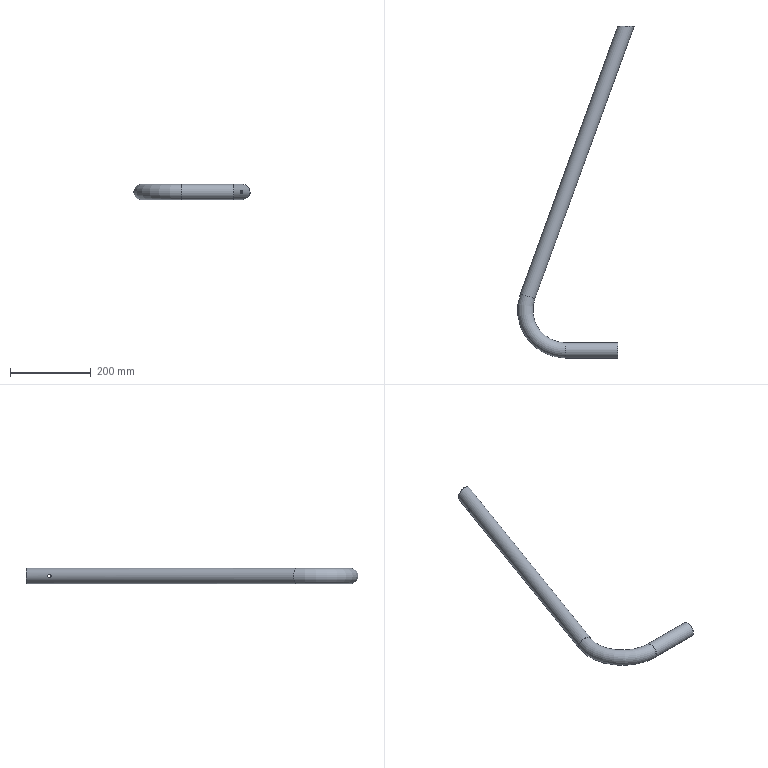Part | STEP file | 6151401 | 1 solid | 10 faces | box 289.236 x 823.315 x 38.1 mm | volume 178322 mm3 | cylinder 6 | torus 2 | plane 2 | commonest cylinder face diameters 9 x2 35.1 x2 38.1 x2
STEP:
#1=CARTESIAN_POINT('',(-23.107,741.765,0.));
#2=VERTEX_POINT('',#1);
#3=CARTESIAN_POINT('',(-23.107,741.765,0.));
#4=CARTESIAN_POINT('',(-23.107,741.765,-0.3084));
#5=CARTESIAN_POINT('',(-23.088,741.797,-0.6103));
#6=CARTESIAN_POINT('',(-23.013,741.918,-1.202));
#7=CARTESIAN_POINT('',(-22.958,742.01,-1.494));
#8=CARTESIAN_POINT('',(-22.819,742.243,-2.039));
#9=CARTESIAN_POINT('',(-22.735,742.384,-2.296));
#10=CARTESIAN_POINT('',(-22.546,742.715,-2.78));
#11=CARTESIAN_POINT('',(-22.443,742.899,-3.));
#12=CARTESIAN_POINT('',(-22.223,743.303,-3.399));
#13=CARTESIAN_POINT('',(-22.106,743.525,-3.581));
#14=CARTESIAN_POINT('',(-21.869,743.992,-3.894));
#15=CARTESIAN_POINT('',(-21.749,744.237,-4.027));
#16=CARTESIAN_POINT('',(-21.51,744.753,-4.248));
#17=CARTESIAN_POINT('',(-21.389,745.024,-4.335));
#18=CARTESIAN_POINT('',(-21.159,745.573,-4.455));
#19=CARTESIAN_POINT('',(-21.048,745.853,-4.49));
#20=CARTESIAN_POINT('',(-20.836,746.425,-4.506));
#21=CARTESIAN_POINT('',(-20.735,746.717,-4.487));
#22=CARTESIAN_POINT('',(-20.551,747.287,-4.392));
#23=CARTESIAN_POINT('',(-20.468,747.569,-4.317));
#24=CARTESIAN_POINT('',(-20.354,747.985,-4.161));
#25=CARTESIAN_POINT('',(-20.318,748.123,-4.101));
#26=CARTESIAN_POINT('',(-20.251,748.39,-3.97));
#27=CARTESIAN_POINT('',(-20.22,748.52,-3.897));
#28=CARTESIAN_POINT('',(-20.133,748.899,-3.661));
#29=CARTESIAN_POINT('',(-20.084,749.138,-3.477));
#30=CARTESIAN_POINT('',(-20.001,749.581,-3.058));
#31=CARTESIAN_POINT('',(-19.968,749.778,-2.829));
#32=CARTESIAN_POINT('',(-19.913,750.125,-2.333));
#33=CARTESIAN_POINT('',(-19.892,750.276,-2.062));
#34=CARTESIAN_POINT('',(-19.86,750.518,-1.503));
#35=CARTESIAN_POINT('',(-19.849,750.609,-1.213));
#36=CARTESIAN_POINT('',(-19.838,750.702,-0.7642));
#37=CARTESIAN_POINT('',(-19.836,750.726,-0.6113));
#38=CARTESIAN_POINT('',(-19.832,750.757,-0.3069));
#39=CARTESIAN_POINT('',(-19.831,750.765,-0.1548));
#40=CARTESIAN_POINT('',(-19.831,750.765,0.301));
#41=CARTESIAN_POINT('',(-19.835,750.735,0.6059));
#42=CARTESIAN_POINT('',(-19.849,750.611,1.208));
#43=CARTESIAN_POINT('',(-19.86,750.52,1.498));
#44=CARTESIAN_POINT('',(-19.892,750.28,2.056));
#45=CARTESIAN_POINT('',(-19.913,750.129,2.327));
#46=CARTESIAN_POINT('',(-19.967,749.782,2.824));
#47=CARTESIAN_POINT('',(-20.,749.585,3.053));
#48=CARTESIAN_POINT('',(-20.083,749.145,3.471));
#49=CARTESIAN_POINT('',(-20.132,748.904,3.658));
#50=CARTESIAN_POINT('',(-20.248,748.398,3.974));
#51=CARTESIAN_POINT('',(-20.315,748.128,4.107));
#52=CARTESIAN_POINT('',(-20.466,747.572,4.316));
#53=CARTESIAN_POINT('',(-20.55,747.29,4.391));
#54=CARTESIAN_POINT('',(-20.735,746.717,4.487));
#55=CARTESIAN_POINT('',(-20.836,746.424,4.506));
#56=CARTESIAN_POINT('',(-21.048,745.853,4.49));
#57=CARTESIAN_POINT('',(-21.159,745.572,4.455));
#58=CARTESIAN_POINT('',(-21.391,745.019,4.333));
#59=CARTESIAN_POINT('',(-21.511,744.749,4.246));
#60=CARTESIAN_POINT('',(-21.75,744.235,4.026));
#61=CARTESIAN_POINT('',(-21.87,743.989,3.892));
#62=CARTESIAN_POINT('',(-22.109,743.519,3.576));
#63=CARTESIAN_POINT('',(-22.224,743.301,3.397));
#64=CARTESIAN_POINT('',(-22.443,742.899,2.999));
#65=CARTESIAN_POINT('',(-22.546,742.715,2.781));
#66=CARTESIAN_POINT('',(-22.735,742.385,2.297));
#67=CARTESIAN_POINT('',(-22.818,742.243,2.04));
#68=CARTESIAN_POINT('',(-22.956,742.012,1.499));
#69=CARTESIAN_POINT('',(-23.012,741.921,1.211));
#70=CARTESIAN_POINT('',(-23.087,741.797,0.6128));
#71=CARTESIAN_POINT('',(-23.107,741.765,0.3084));
#72=CARTESIAN_POINT('',(-23.107,741.765,0.));
#73=B_SPLINE_CURVE_WITH_KNOTS('',3,(#3,#4,#5,#6,#7,#8,#9,#10,#11,#12,#13,#14,#15,#16,#17,#18,#19,#20,#21,#22,#23,#24,#25,#26,#27,#28,#29,#30,#31,#32,#33,#34,#35,#36,#37,#38,#39,#40,#41,#42,#43,#44,#45,#46,#47,#48,#49,#50,#51,#52,#53,#54,#55,#56,#57,#58,#59,#60,#61,#62,#63,#64,#65,#66,#67,#68,#69,#70,#71,#72),.UNSPECIFIED.,.T.,.F.,(4,2,2,2,2,2,2,2,2,2,2,2,2,2,2,2,2,2,2,2,2,2,2,2,2,2,2,2,2,2,2,2,2,2,4),(0.,0.0009109,0.001822,0.002733,0.003644,0.004555,0.005465,0.006376,0.007287,0.008198,0.009109,0.009564,0.01002,0.01093,0.01184,0.01275,0.01366,0.01412,0.01457,0.01549,0.0164,0.01731,0.01822,0.01913,0.02004,0.02095,0.02186,0.02277,0.02368,0.02459,0.02551,0.02642,0.02733,0.02824,0.02915),.UNSPECIFIED.);
#74=EDGE_CURVE('',#2,#2,#73,.T.);
#75=ORIENTED_EDGE('',*,*,#74,.T.);
#76=EDGE_LOOP('',(#75));
#77=FACE_BOUND('',#76,.T.);
#78=CARTESIAN_POINT('',(17.438,741.765,0.));
#79=VERTEX_POINT('',#78);
#80=CARTESIAN_POINT('',(17.438,741.765,0.));
#81=CARTESIAN_POINT('',(17.438,741.765,0.3079));
#82=CARTESIAN_POINT('',(17.442,741.796,0.6104));
#83=CARTESIAN_POINT('',(17.456,741.919,1.205));
#84=CARTESIAN_POINT('',(17.467,742.012,1.501));
#85=CARTESIAN_POINT('',(17.499,742.253,2.06));
#86=CARTESIAN_POINT('',(17.52,742.4,2.325));
#87=CARTESIAN_POINT('',(17.574,742.748,2.824));
#88=CARTESIAN_POINT('',(17.608,742.949,3.057));
#89=CARTESIAN_POINT('',(17.69,743.385,3.471));
#90=CARTESIAN_POINT('',(17.739,743.624,3.656));
#91=CARTESIAN_POINT('',(17.855,744.135,3.976));
#92=CARTESIAN_POINT('',(17.922,744.402,4.107));
#93=CARTESIAN_POINT('',(18.072,744.953,4.314));
#94=CARTESIAN_POINT('',(18.157,745.241,4.391));
#95=CARTESIAN_POINT('',(18.342,745.814,4.487));
#96=CARTESIAN_POINT('',(18.441,746.101,4.506));
#97=CARTESIAN_POINT('',(18.653,746.674,4.491));
#98=CARTESIAN_POINT('',(18.766,746.958,4.455));
#99=CARTESIAN_POINT('',(18.997,747.507,4.334));
#100=CARTESIAN_POINT('',(19.115,747.774,4.249));
#101=CARTESIAN_POINT('',(19.478,748.554,3.916));
#102=CARTESIAN_POINT('',(19.717,749.019,3.605));
#103=CARTESIAN_POINT('',(20.049,749.631,3.001));
#104=CARTESIAN_POINT('',(20.152,749.814,2.782));
#105=CARTESIAN_POINT('',(20.339,750.139,2.307));
#106=CARTESIAN_POINT('',(20.423,750.282,2.05));
#107=CARTESIAN_POINT('',(20.563,750.518,1.501));
#108=CARTESIAN_POINT('',(20.618,750.608,1.216));
#109=CARTESIAN_POINT('',(20.674,750.7,0.7752));
#110=CARTESIAN_POINT('',(20.689,750.724,0.6257));
#111=CARTESIAN_POINT('',(20.709,750.756,0.3212));
#112=CARTESIAN_POINT('',(20.714,750.765,0.1668));
#113=CARTESIAN_POINT('',(20.715,750.766,-0.2909));
#114=CARTESIAN_POINT('',(20.696,750.736,-0.5928));
#115=CARTESIAN_POINT('',(20.622,750.616,-1.191));
#116=CARTESIAN_POINT('',(20.568,750.525,-1.48));
#117=CARTESIAN_POINT('',(20.429,750.294,-2.027));
#118=CARTESIAN_POINT('',(20.345,750.15,-2.289));
#119=CARTESIAN_POINT('',(20.158,749.824,-2.77));
#120=CARTESIAN_POINT('',(20.054,749.64,-2.99));
#121=CARTESIAN_POINT('',(19.833,749.233,-3.395));
#122=CARTESIAN_POINT('',(19.717,749.014,-3.574));
#123=CARTESIAN_POINT('',(19.481,748.549,-3.888));
#124=CARTESIAN_POINT('',(19.36,748.3,-4.023));
#125=CARTESIAN_POINT('',(19.119,747.783,-4.246));
#126=CARTESIAN_POINT('',(19.,747.516,-4.332));
#127=CARTESIAN_POINT('',(18.77,746.968,-4.454));
#128=CARTESIAN_POINT('',(18.657,746.682,-4.49));
#129=CARTESIAN_POINT('',(18.444,746.109,-4.506));
#130=CARTESIAN_POINT('',(18.345,745.823,-4.488));
#131=CARTESIAN_POINT('',(18.161,745.252,-4.394));
#132=CARTESIAN_POINT('',(18.075,744.964,-4.318));
#133=CARTESIAN_POINT('',(17.924,744.41,-4.11));
#134=CARTESIAN_POINT('',(17.857,744.144,-3.98));
#135=CARTESIAN_POINT('',(17.741,743.636,-3.665));
#136=CARTESIAN_POINT('',(17.691,743.393,-3.477));
#137=CARTESIAN_POINT('',(17.609,742.955,-3.063));
#138=CARTESIAN_POINT('',(17.575,742.757,-2.834));
#139=CARTESIAN_POINT('',(17.52,742.405,-2.333));
#140=CARTESIAN_POINT('',(17.499,742.256,-2.065));
#141=CARTESIAN_POINT('',(17.468,742.015,-1.508));
#142=CARTESIAN_POINT('',(17.456,741.921,-1.214));
#143=CARTESIAN_POINT('',(17.442,741.797,-0.6129));
#144=CARTESIAN_POINT('',(17.438,741.765,-0.3079));
#145=CARTESIAN_POINT('',(17.438,741.765,0.));
#146=B_SPLINE_CURVE_WITH_KNOTS('',3,(#80,#81,#82,#83,#84,#85,#86,#87,#88,#89,#90,#91,#92,#93,#94,#95,#96,#97,#98,#99,#100,#101,#102,#103,#104,#105,#106,#107,#108,#109,#110,#111,#112,#113,#114,#115,#116,#117,#118,#119,#120,#121,#122,#123,#124,#125,#126,#127,#128,#129,#130,#131,#132,#133,#134,#135,#136,#137,#138,#139,#140,#141,#142,#143,#144,#145),.UNSPECIFIED.,.T.,.F.,(4,2,2,2,2,2,2,2,2,2,2,2,2,2,2,2,2,2,2,2,2,2,2,2,2,2,2,2,2,2,2,2,4),(0.,0.0009106,0.001821,0.002732,0.003642,0.004553,0.005464,0.006374,0.007285,0.008196,0.009106,0.01093,0.01184,0.01275,0.01366,0.01411,0.01457,0.01548,0.01639,0.0173,0.01821,0.01912,0.02003,0.02094,0.02185,0.02277,0.02368,0.02459,0.0255,0.02641,0.02732,0.02823,0.02914),.UNSPECIFIED.);
#147=EDGE_CURVE('',#79,#79,#146,.T.);
#148=ORIENTED_EDGE('',*,*,#147,.T.);
#149=EDGE_LOOP('',(#148));
#150=FACE_BOUND('',#149,.T.);
#151=CARTESIAN_POINT('',(40.186,804.265,0.));
#152=VERTEX_POINT('',#151);
#153=CARTESIAN_POINT('',(40.186,804.265,0.));
#154=CARTESIAN_POINT('',(40.186,804.265,38.1));
#155=CARTESIAN_POINT('',(-0.3588,804.265,38.1));
#156=CARTESIAN_POINT('',(-0.3588,804.265,0.));
#157=CARTESIAN_POINT('',(-0.3588,804.265,-38.1));
#158=CARTESIAN_POINT('',(40.186,804.265,-38.1));
#159=CARTESIAN_POINT('',(40.186,804.265,0.));
#160=(BOUNDED_CURVE()B_SPLINE_CURVE(3,(#153,#154,#155,#156,#157,#158,#159),.UNSPECIFIED.,.T.,.F.)B_SPLINE_CURVE_WITH_KNOTS((4,3,4),(0.,3.142,6.283),.UNSPECIFIED.)CURVE()GEOMETRIC_REPRESENTATION_ITEM()RATIONAL_B_SPLINE_CURVE((1.,0.3333,0.3333,1.,0.3333,0.3333,1.))REPRESENTATION_ITEM(''));
#161=EDGE_CURVE('',#152,#152,#160,.T.);
#162=ORIENTED_EDGE('',*,*,#161,.T.);
#163=EDGE_LOOP('',(#162));
#164=FACE_OUTER_BOUND('',#163,.T.);
#165=CARTESIAN_POINT('',(-223.969,134.202,-19.05));
#166=VERTEX_POINT('',#165);
#167=CARTESIAN_POINT('',(-223.969,134.202,0.));
#168=DIRECTION('',(-0.342,-0.9397,0.));
#169=DIRECTION('',(0.,0.,-1.));
#170=AXIS2_PLACEMENT_3D('',#167,#168,#169);
#171=CIRCLE('',#170,19.05);
#172=EDGE_CURVE('',#166,#166,#171,.T.);
#173=ORIENTED_EDGE('',*,*,#172,.F.);
#174=EDGE_LOOP('',(#173));
#175=FACE_OUTER_BOUND('',#174,.T.);
#176=CARTESIAN_POINT('',(-223.969,134.202,0.));
#177=DIRECTION('',(0.342,0.9397,0.));
#178=DIRECTION('',(-0.9397,0.342,0.));
#179=AXIS2_PLACEMENT_3D('',#176,#177,#178);
#180=CYLINDRICAL_SURFACE('',#179,19.05);
#181=ADVANCED_FACE('',(#77,#150,#164,#175),#180,.T.);
#182=CARTESIAN_POINT('',(-21.511,741.765,0.));
#183=VERTEX_POINT('',#182);
#184=CARTESIAN_POINT('',(-21.511,741.765,0.));
#185=CARTESIAN_POINT('',(-21.511,741.765,-0.3086));
#186=CARTESIAN_POINT('',(-21.491,741.797,-0.6106));
#187=CARTESIAN_POINT('',(-21.414,741.918,-1.202));
#188=CARTESIAN_POINT('',(-21.356,742.01,-1.494));
#189=CARTESIAN_POINT('',(-21.213,742.243,-2.039));
#190=CARTESIAN_POINT('',(-21.127,742.384,-2.296));
#191=CARTESIAN_POINT('',(-20.932,742.713,-2.778));
#192=CARTESIAN_POINT('',(-20.826,742.897,-2.997));
#193=CARTESIAN_POINT('',(-20.601,743.299,-3.396));
#194=CARTESIAN_POINT('',(-20.481,743.52,-3.577));
#195=CARTESIAN_POINT('',(-20.239,743.985,-3.89));
#196=CARTESIAN_POINT('',(-20.117,744.229,-4.023));
#197=CARTESIAN_POINT('',(-19.873,744.743,-4.244));
#198=CARTESIAN_POINT('',(-19.751,745.014,-4.332));
#199=CARTESIAN_POINT('',(-19.518,745.562,-4.454));
#200=CARTESIAN_POINT('',(-19.406,745.841,-4.489));
#201=CARTESIAN_POINT('',(-19.193,746.413,-4.507));
#202=CARTESIAN_POINT('',(-19.092,746.705,-4.488));
#203=CARTESIAN_POINT('',(-18.91,747.277,-4.394));
#204=CARTESIAN_POINT('',(-18.828,747.559,-4.32));
#205=CARTESIAN_POINT('',(-18.717,747.976,-4.165));
#206=CARTESIAN_POINT('',(-18.682,748.115,-4.105));
#207=CARTESIAN_POINT('',(-18.617,748.383,-3.973));
#208=CARTESIAN_POINT('',(-18.588,748.513,-3.901));
#209=CARTESIAN_POINT('',(-18.505,748.894,-3.665));
#210=CARTESIAN_POINT('',(-18.459,749.133,-3.481));
#211=CARTESIAN_POINT('',(-18.382,749.578,-3.061));
#212=CARTESIAN_POINT('',(-18.352,749.775,-2.832));
#213=CARTESIAN_POINT('',(-18.304,750.124,-2.335));
#214=CARTESIAN_POINT('',(-18.286,750.275,-2.065));
#215=CARTESIAN_POINT('',(-18.259,750.517,-1.505));
#216=CARTESIAN_POINT('',(-18.25,750.609,-1.215));
#217=CARTESIAN_POINT('',(-18.238,750.733,-0.6156));
#218=CARTESIAN_POINT('',(-18.235,750.765,-0.3081));
#219=CARTESIAN_POINT('',(-18.235,750.765,0.2999));
#220=CARTESIAN_POINT('',(-18.238,750.735,0.6057));
#221=CARTESIAN_POINT('',(-18.25,750.611,1.207));
#222=CARTESIAN_POINT('',(-18.259,750.52,1.497));
#223=CARTESIAN_POINT('',(-18.285,750.279,2.056));
#224=CARTESIAN_POINT('',(-18.304,750.128,2.328));
#225=CARTESIAN_POINT('',(-18.352,749.781,2.826));
#226=CARTESIAN_POINT('',(-18.381,749.583,3.055));
#227=CARTESIAN_POINT('',(-18.458,749.142,3.474));
#228=CARTESIAN_POINT('',(-18.504,748.9,3.66));
#229=CARTESIAN_POINT('',(-18.613,748.393,3.977));
#230=CARTESIAN_POINT('',(-18.678,748.122,4.11));
#231=CARTESIAN_POINT('',(-18.826,747.565,4.318));
#232=CARTESIAN_POINT('',(-18.908,747.282,4.393));
#233=CARTESIAN_POINT('',(-19.091,746.707,4.488));
#234=CARTESIAN_POINT('',(-19.192,746.414,4.507));
#235=CARTESIAN_POINT('',(-19.405,745.844,4.489));
#236=CARTESIAN_POINT('',(-19.517,745.563,4.454));
#237=CARTESIAN_POINT('',(-19.752,745.01,4.331));
#238=CARTESIAN_POINT('',(-19.874,744.741,4.243));
#239=CARTESIAN_POINT('',(-20.117,744.229,4.023));
#240=CARTESIAN_POINT('',(-20.24,743.984,3.889));
#241=CARTESIAN_POINT('',(-20.483,743.515,3.573));
#242=CARTESIAN_POINT('',(-20.601,743.298,3.395));
#243=CARTESIAN_POINT('',(-20.825,742.898,2.998));
#244=CARTESIAN_POINT('',(-20.931,742.714,2.779));
#245=CARTESIAN_POINT('',(-21.126,742.384,2.297));
#246=CARTESIAN_POINT('',(-21.212,742.244,2.04));
#247=CARTESIAN_POINT('',(-21.356,742.011,1.496));
#248=CARTESIAN_POINT('',(-21.413,741.919,1.204));
#249=CARTESIAN_POINT('',(-21.491,741.797,0.6114));
#250=CARTESIAN_POINT('',(-21.511,741.765,0.3086));
#251=CARTESIAN_POINT('',(-21.511,741.765,0.));
#252=B_SPLINE_CURVE_WITH_KNOTS('',3,(#184,#185,#186,#187,#188,#189,#190,#191,#192,#193,#194,#195,#196,#197,#198,#199,#200,#201,#202,#203,#204,#205,#206,#207,#208,#209,#210,#211,#212,#213,#214,#215,#216,#217,#218,#219,#220,#221,#222,#223,#224,#225,#226,#227,#228,#229,#230,#231,#232,#233,#234,#235,#236,#237,#238,#239,#240,#241,#242,#243,#244,#245,#246,#247,#248,#249,#250,#251),.UNSPECIFIED.,.T.,.F.,(4,2,2,2,2,2,2,2,2,2,2,2,2,2,2,2,2,2,2,2,2,2,2,2,2,2,2,2,2,2,2,2,2,4),(0.,0.0009114,0.001823,0.002734,0.003646,0.004557,0.005468,0.00638,0.007291,0.008202,0.009114,0.009569,0.01003,0.01094,0.01185,0.01276,0.01367,0.01458,0.01549,0.0164,0.01732,0.01823,0.01914,0.02005,0.02096,0.02187,0.02278,0.0237,0.02461,0.02552,0.02643,0.02734,0.02825,0.02916),.UNSPECIFIED.);
#253=EDGE_CURVE('',#183,#183,#252,.T.);
#254=ORIENTED_EDGE('',*,*,#253,.F.);
#255=EDGE_LOOP('',(#254));
#256=FACE_BOUND('',#255,.T.);
#257=CARTESIAN_POINT('',(15.842,741.765,0.));
#258=VERTEX_POINT('',#257);
#259=CARTESIAN_POINT('',(15.842,741.765,0.));
#260=CARTESIAN_POINT('',(15.842,741.765,0.3081));
#261=CARTESIAN_POINT('',(15.845,741.797,0.6108));
#262=CARTESIAN_POINT('',(15.857,741.919,1.206));
#263=CARTESIAN_POINT('',(15.866,742.012,1.502));
#264=CARTESIAN_POINT('',(15.893,742.254,2.061));
#265=CARTESIAN_POINT('',(15.911,742.401,2.326));
#266=CARTESIAN_POINT('',(15.959,742.75,2.826));
#267=CARTESIAN_POINT('',(15.989,742.951,3.059));
#268=CARTESIAN_POINT('',(16.065,743.389,3.474));
#269=CARTESIAN_POINT('',(16.11,743.628,3.659));
#270=CARTESIAN_POINT('',(16.221,744.141,3.979));
#271=CARTESIAN_POINT('',(16.285,744.408,4.11));
#272=CARTESIAN_POINT('',(16.432,744.961,4.317));
#273=CARTESIAN_POINT('',(16.516,745.25,4.394));
#274=CARTESIAN_POINT('',(16.698,745.824,4.488));
#275=CARTESIAN_POINT('',(16.797,746.111,4.506));
#276=CARTESIAN_POINT('',(17.011,746.684,4.49));
#277=CARTESIAN_POINT('',(17.125,746.968,4.454));
#278=CARTESIAN_POINT('',(17.358,747.517,4.332));
#279=CARTESIAN_POINT('',(17.478,747.783,4.246));
#280=CARTESIAN_POINT('',(17.724,748.301,4.023));
#281=CARTESIAN_POINT('',(17.846,748.546,3.889));
#282=CARTESIAN_POINT('',(18.087,749.008,3.578));
#283=CARTESIAN_POINT('',(18.205,749.227,3.4));
#284=CARTESIAN_POINT('',(18.432,749.632,2.999));
#285=CARTESIAN_POINT('',(18.538,749.815,2.781));
#286=CARTESIAN_POINT('',(18.73,750.139,2.307));
#287=CARTESIAN_POINT('',(18.816,750.282,2.05));
#288=CARTESIAN_POINT('',(18.961,750.518,1.502));
#289=CARTESIAN_POINT('',(19.018,750.608,1.218));
#290=CARTESIAN_POINT('',(19.076,750.7,0.7769));
#291=CARTESIAN_POINT('',(19.091,750.724,0.6274));
#292=CARTESIAN_POINT('',(19.112,750.756,0.3228));
#293=CARTESIAN_POINT('',(19.117,750.765,0.1682));
#294=CARTESIAN_POINT('',(19.118,750.766,-0.2897));
#295=CARTESIAN_POINT('',(19.099,750.737,-0.5918));
#296=CARTESIAN_POINT('',(19.023,750.616,-1.19));
#297=CARTESIAN_POINT('',(18.966,750.526,-1.479));
#298=CARTESIAN_POINT('',(18.824,750.294,-2.026));
#299=CARTESIAN_POINT('',(18.737,750.151,-2.287));
#300=CARTESIAN_POINT('',(18.544,749.826,-2.767));
#301=CARTESIAN_POINT('',(18.438,749.643,-2.987));
#302=CARTESIAN_POINT('',(18.211,749.237,-3.391));
#303=CARTESIAN_POINT('',(18.092,749.019,-3.57));
#304=CARTESIAN_POINT('',(17.851,748.556,-3.884));
#305=CARTESIAN_POINT('',(17.727,748.308,-4.019));
#306=CARTESIAN_POINT('',(17.482,747.792,-4.242));
#307=CARTESIAN_POINT('',(17.362,747.527,-4.329));
#308=CARTESIAN_POINT('',(17.129,746.979,-4.452));
#309=CARTESIAN_POINT('',(17.015,746.694,-4.489));
#310=CARTESIAN_POINT('',(16.801,746.121,-4.507));
#311=CARTESIAN_POINT('',(16.702,745.835,-4.489));
#312=CARTESIAN_POINT('',(16.52,745.263,-4.396));
#313=CARTESIAN_POINT('',(16.435,744.974,-4.321));
#314=CARTESIAN_POINT('',(16.287,744.418,-4.114));
#315=CARTESIAN_POINT('',(16.224,744.151,-3.984));
#316=CARTESIAN_POINT('',(16.113,743.641,-3.668));
#317=CARTESIAN_POINT('',(16.066,743.397,-3.481));
#318=CARTESIAN_POINT('',(15.99,742.957,-3.066));
#319=CARTESIAN_POINT('',(15.96,742.759,-2.837));
#320=CARTESIAN_POINT('',(15.911,742.406,-2.335));
#321=CARTESIAN_POINT('',(15.893,742.257,-2.067));
#322=CARTESIAN_POINT('',(15.866,742.015,-1.509));
#323=CARTESIAN_POINT('',(15.857,741.921,-1.214));
#324=CARTESIAN_POINT('',(15.845,741.797,-0.6132));
#325=CARTESIAN_POINT('',(15.842,741.765,-0.3081));
#326=CARTESIAN_POINT('',(15.842,741.765,0.));
#327=B_SPLINE_CURVE_WITH_KNOTS('',3,(#259,#260,#261,#262,#263,#264,#265,#266,#267,#268,#269,#270,#271,#272,#273,#274,#275,#276,#277,#278,#279,#280,#281,#282,#283,#284,#285,#286,#287,#288,#289,#290,#291,#292,#293,#294,#295,#296,#297,#298,#299,#300,#301,#302,#303,#304,#305,#306,#307,#308,#309,#310,#311,#312,#313,#314,#315,#316,#317,#318,#319,#320,#321,#322,#323,#324,#325,#326),.UNSPECIFIED.,.T.,.F.,(4,2,2,2,2,2,2,2,2,2,2,2,2,2,2,2,2,2,2,2,2,2,2,2,2,2,2,2,2,2,2,2,2,4),(0.,0.0009111,0.001822,0.002733,0.003644,0.004556,0.005467,0.006378,0.007289,0.0082,0.009111,0.01002,0.01093,0.01184,0.01276,0.01367,0.01412,0.01458,0.01549,0.0164,0.01731,0.01822,0.01913,0.02004,0.02096,0.02187,0.02278,0.02369,0.0246,0.02551,0.02642,0.02733,0.02824,0.02916),.UNSPECIFIED.);
#328=EDGE_CURVE('',#258,#258,#327,.T.);
#329=ORIENTED_EDGE('',*,*,#328,.F.);
#330=EDGE_LOOP('',(#329));
#331=FACE_BOUND('',#330,.T.);
#332=CARTESIAN_POINT('',(38.59,804.265,0.));
#333=VERTEX_POINT('',#332);
#334=CARTESIAN_POINT('',(38.59,804.265,0.));
#335=CARTESIAN_POINT('',(38.59,804.265,35.1));
#336=CARTESIAN_POINT('',(1.237,804.265,35.1));
#337=CARTESIAN_POINT('',(1.237,804.265,0.));
#338=CARTESIAN_POINT('',(1.237,804.265,-35.1));
#339=CARTESIAN_POINT('',(38.59,804.265,-35.1));
#340=CARTESIAN_POINT('',(38.59,804.265,0.));
#341=(BOUNDED_CURVE()B_SPLINE_CURVE(3,(#334,#335,#336,#337,#338,#339,#340),.UNSPECIFIED.,.T.,.T.)B_SPLINE_CURVE_WITH_KNOTS((4,3,4),(0.,3.142,6.283),.UNSPECIFIED.)CURVE()GEOMETRIC_REPRESENTATION_ITEM()RATIONAL_B_SPLINE_CURVE((1.,0.3333,0.3333,1.,0.3333,0.3333,1.))REPRESENTATION_ITEM(''));
#342=EDGE_CURVE('',#333,#333,#341,.T.);
#343=ORIENTED_EDGE('',*,*,#342,.F.);
#344=EDGE_LOOP('',(#343));
#345=FACE_OUTER_BOUND('',#344,.T.);
#346=CARTESIAN_POINT('',(-223.969,134.202,-17.55));
#347=VERTEX_POINT('',#346);
#348=CARTESIAN_POINT('',(-223.969,134.202,0.));
#349=DIRECTION('',(-0.342,-0.9397,0.));
#350=DIRECTION('',(0.,0.,-1.));
#351=AXIS2_PLACEMENT_3D('',#348,#349,#350);
#352=CIRCLE('',#351,17.55);
#353=EDGE_CURVE('',#347,#347,#352,.T.);
#354=ORIENTED_EDGE('',*,*,#353,.T.);
#355=EDGE_LOOP('',(#354));
#356=FACE_OUTER_BOUND('',#355,.T.);
#357=CARTESIAN_POINT('',(-223.969,134.202,0.));
#358=DIRECTION('',(0.342,0.9397,0.));
#359=DIRECTION('',(-0.9397,0.342,0.));
#360=AXIS2_PLACEMENT_3D('',#357,#358,#359);
#361=CYLINDRICAL_SURFACE('',#360,17.55);
#362=ADVANCED_FACE('',(#256,#331,#345,#356),#361,.F.);
#363=CARTESIAN_POINT('',(-130.,0.,-19.05));
#364=VERTEX_POINT('',#363);
#365=CARTESIAN_POINT('',(-130.,0.,0.));
#366=DIRECTION('',(1.,0.,0.));
#367=DIRECTION('',(0.,0.,-1.));
#368=AXIS2_PLACEMENT_3D('',#365,#366,#367);
#369=CIRCLE('',#368,19.05);
#370=EDGE_CURVE('',#364,#364,#369,.T.);
#371=ORIENTED_EDGE('',*,*,#370,.F.);
#372=EDGE_LOOP('',(#371));
#373=FACE_OUTER_BOUND('',#372,.T.);
#374=ORIENTED_EDGE('',*,*,#172,.T.);
#375=EDGE_LOOP('',(#374));
#376=FACE_OUTER_BOUND('',#375,.T.);
#377=CARTESIAN_POINT('',(-130.,100.,0.));
#378=DIRECTION('',(0.,0.,-1.));
#379=DIRECTION('',(-1.,0.,0.));
#380=AXIS2_PLACEMENT_3D('',#377,#378,#379);
#381=TOROIDAL_SURFACE('',#380,100.,19.05);
#382=ADVANCED_FACE('',(#373,#376),#381,.T.);
#383=CARTESIAN_POINT('',(-130.,0.,-17.55));
#384=VERTEX_POINT('',#383);
#385=CARTESIAN_POINT('',(-130.,0.,0.));
#386=DIRECTION('',(1.,0.,0.));
#387=DIRECTION('',(0.,0.,-1.));
#388=AXIS2_PLACEMENT_3D('',#385,#386,#387);
#389=CIRCLE('',#388,17.55);
#390=EDGE_CURVE('',#384,#384,#389,.T.);
#391=ORIENTED_EDGE('',*,*,#390,.T.);
#392=EDGE_LOOP('',(#391));
#393=FACE_OUTER_BOUND('',#392,.T.);
#394=ORIENTED_EDGE('',*,*,#353,.F.);
#395=EDGE_LOOP('',(#394));
#396=FACE_OUTER_BOUND('',#395,.T.);
#397=CARTESIAN_POINT('',(-130.,100.,0.));
#398=DIRECTION('',(0.,0.,-1.));
#399=DIRECTION('',(-1.,0.,0.));
#400=AXIS2_PLACEMENT_3D('',#397,#398,#399);
#401=TOROIDAL_SURFACE('',#400,100.,17.55);
#402=ADVANCED_FACE('',(#393,#396),#401,.F.);
#403=ORIENTED_EDGE('',*,*,#390,.F.);
#404=EDGE_LOOP('',(#403));
#405=FACE_OUTER_BOUND('',#404,.T.);
#406=CARTESIAN_POINT('',(0.,0.,-17.55));
#407=VERTEX_POINT('',#406);
#408=CARTESIAN_POINT('',(0.,0.,0.));
#409=DIRECTION('',(1.,0.,0.));
#410=DIRECTION('',(0.,0.,-1.));
#411=AXIS2_PLACEMENT_3D('',#408,#409,#410);
#412=CIRCLE('',#411,17.55);
#413=EDGE_CURVE('',#407,#407,#412,.T.);
#414=ORIENTED_EDGE('',*,*,#413,.T.);
#415=EDGE_LOOP('',(#414));
#416=FACE_OUTER_BOUND('',#415,.T.);
#417=CARTESIAN_POINT('',(-130.,0.,0.));
#418=DIRECTION('',(1.,0.,0.));
#419=DIRECTION('',(0.,0.,-1.));
#420=AXIS2_PLACEMENT_3D('',#417,#418,#419);
#421=CYLINDRICAL_SURFACE('',#420,17.55);
#422=ADVANCED_FACE('',(#405,#416),#421,.F.);
#423=ORIENTED_EDGE('',*,*,#370,.T.);
#424=EDGE_LOOP('',(#423));
#425=FACE_OUTER_BOUND('',#424,.T.);
#426=CARTESIAN_POINT('',(0.,0.,-19.05));
#427=VERTEX_POINT('',#426);
#428=CARTESIAN_POINT('',(0.,0.,0.));
#429=DIRECTION('',(1.,0.,0.));
#430=DIRECTION('',(0.,0.,-1.));
#431=AXIS2_PLACEMENT_3D('',#428,#429,#430);
#432=CIRCLE('',#431,19.05);
#433=EDGE_CURVE('',#427,#427,#432,.T.);
#434=ORIENTED_EDGE('',*,*,#433,.F.);
#435=EDGE_LOOP('',(#434));
#436=FACE_OUTER_BOUND('',#435,.T.);
#437=CARTESIAN_POINT('',(-130.,0.,0.));
#438=DIRECTION('',(1.,0.,0.));
#439=DIRECTION('',(0.,0.,-1.));
#440=AXIS2_PLACEMENT_3D('',#437,#438,#439);
#441=CYLINDRICAL_SURFACE('',#440,19.05);
#442=ADVANCED_FACE('',(#425,#436),#441,.T.);
#443=ORIENTED_EDGE('',*,*,#413,.F.);
#444=EDGE_LOOP('',(#443));
#445=FACE_BOUND('',#444,.T.);
#446=ORIENTED_EDGE('',*,*,#433,.T.);
#447=EDGE_LOOP('',(#446));
#448=FACE_OUTER_BOUND('',#447,.T.);
#449=CARTESIAN_POINT('',(0.,0.,0.));
#450=DIRECTION('',(1.,0.,0.));
#451=DIRECTION('',(0.,0.,-1.));
#452=AXIS2_PLACEMENT_3D('',#449,#450,#451);
#453=PLANE('',#452);
#454=ADVANCED_FACE('',(#445,#448),#453,.T.);
#455=ORIENTED_EDGE('',*,*,#342,.T.);
#456=EDGE_LOOP('',(#455));
#457=FACE_BOUND('',#456,.T.);
#458=ORIENTED_EDGE('',*,*,#161,.F.);
#459=EDGE_LOOP('',(#458));
#460=FACE_OUTER_BOUND('',#459,.T.);
#461=CARTESIAN_POINT('',(40.186,804.265,1131.022));
#462=DIRECTION('',(0.,-1.,0.));
#463=DIRECTION('',(0.,0.,-1.));
#464=AXIS2_PLACEMENT_3D('',#461,#462,#463);
#465=PLANE('',#464);
#466=ADVANCED_FACE('',(#457,#460),#465,.F.);
#467=ORIENTED_EDGE('',*,*,#328,.T.);
#468=EDGE_LOOP('',(#467));
#469=FACE_OUTER_BOUND('',#468,.T.);
#470=ORIENTED_EDGE('',*,*,#147,.F.);
#471=EDGE_LOOP('',(#470));
#472=FACE_OUTER_BOUND('',#471,.T.);
#473=CARTESIAN_POINT('',(92.51,746.265,0.));
#474=DIRECTION('',(-1.,0.,0.));
#475=DIRECTION('',(0.,-1.,0.));
#476=AXIS2_PLACEMENT_3D('',#473,#474,#475);
#477=CYLINDRICAL_SURFACE('',#476,4.5);
#478=ADVANCED_FACE('',(#469,#472),#477,.F.);
#479=ORIENTED_EDGE('',*,*,#253,.T.);
#480=EDGE_LOOP('',(#479));
#481=FACE_OUTER_BOUND('',#480,.T.);
#482=ORIENTED_EDGE('',*,*,#74,.F.);
#483=EDGE_LOOP('',(#482));
#484=FACE_OUTER_BOUND('',#483,.T.);
#485=CARTESIAN_POINT('',(92.51,746.265,0.));
#486=DIRECTION('',(-1.,0.,0.));
#487=DIRECTION('',(0.,-1.,0.));
#488=AXIS2_PLACEMENT_3D('',#485,#486,#487);
#489=CYLINDRICAL_SURFACE('',#488,4.5);
#490=ADVANCED_FACE('',(#481,#484),#489,.F.);
#491=CLOSED_SHELL('',(#181,#362,#382,#402,#422,#442,#454,#466,#478,#490));
#492=MANIFOLD_SOLID_BREP('',#491);
#493=CARTESIAN_POINT('',(0.,0.,0.));
#494=DIRECTION('',(0.,0.,1.));
#495=DIRECTION('',(1.,0.,0.));
#496=AXIS2_PLACEMENT_3D('',#493,#494,#495);
#497=(LENGTH_UNIT()NAMED_UNIT(*)SI_UNIT(.MILLI.,.METRE.));
#498=UNCERTAINTY_MEASURE_WITH_UNIT(LENGTH_MEASURE(0.00001),#497,'','');
#499=(NAMED_UNIT(*)PLANE_ANGLE_UNIT()SI_UNIT($,.RADIAN.));
#500=(NAMED_UNIT(*)SI_UNIT($,.STERADIAN.)SOLID_ANGLE_UNIT());
#501=(GEOMETRIC_REPRESENTATION_CONTEXT(3)GLOBAL_UNCERTAINTY_ASSIGNED_CONTEXT((#498))GLOBAL_UNIT_ASSIGNED_CONTEXT((#497,#499,#500))REPRESENTATION_CONTEXT('',''));
#502=ADVANCED_BREP_SHAPE_REPRESENTATION('',(#492,#496),#501);